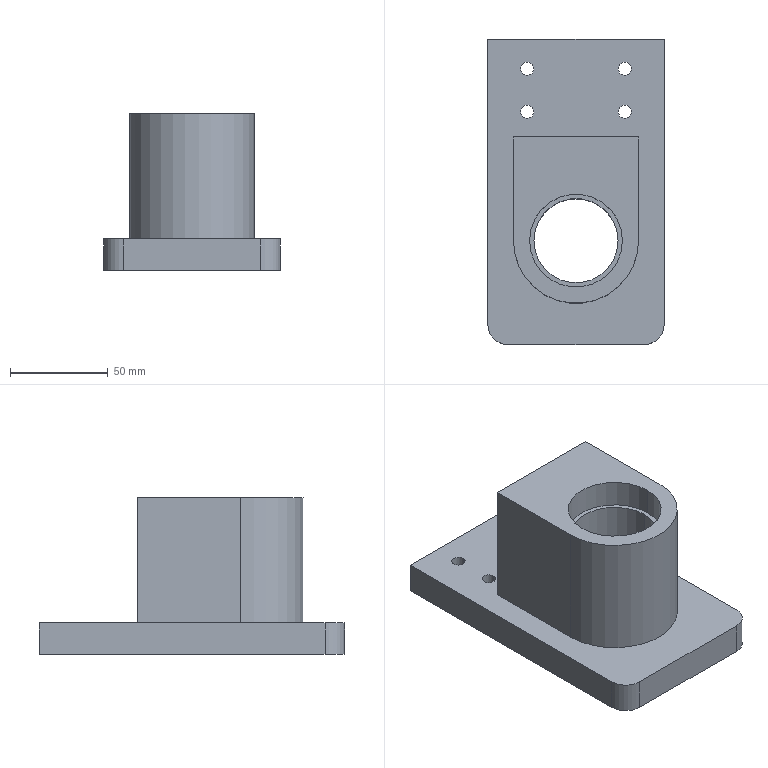NC program | NX | posted with a generic post | part box 90 x 156 x 80 mm
Lines 1 to 1164 of 8711:
N10 G17 G21 G94 G90
(CAVITY_MILL_COPY , TOOL : 刀杆C25-D25-150-2T)
N12 T01 M6
N14 G53
N16 G17 G0 G90 X-98.941 Y0. S2000 M3
N18 G43 Z30. H1
N20 Z1.5
N22 G94 G1 Z-0.5 F3000.
N24 X-82.691
N26 Y48.791
N28 X-82.682 Y50.031
N30 G2 X-81.523 Y51.183 R1.159
N32 G1 X81.523
N34 G2 X82.682 Y50.031 R1.159
N36 G1 X82.691 Y48.791
N38 Y28.521
N40 X63.971
N42 G3 X60.754 Y32.463 R48.293
N44 G1 X63.971
N46 Y28.521
N48 X70.565 Y17.419
N50 X63.971 Y28.521
N52 X82.691
N54 Y-48.791
N56 X82.682 Y-50.031
N58 G2 X81.523 Y-51.183 R1.159
N60 G1 X60.754
N62 Y-32.463
N64 G3 X63.971 Y-28.521 R48.293
N66 G1 X70.565 Y-17.419
N68 X63.971 Y-28.521
N70 Y-32.463
N72 X60.754
N74 Y-51.183
N76 X-81.523
N78 G2 X-82.682 Y-50.031 R1.159
N80 G1 X-82.691 Y-48.791
N82 Y0.
N84 X-63.971
N86 Y32.463
N88 X-44.264
N90 G3 X-44.293 Y32. R3.744
N92 G1 Y-32.
N94 G3 X-44.264 Y-32.463 R3.744
N96 G1 X-40.549 Y-32.
N98 Y32.
N100 X-40.532 Y32.037
N102 X-40.47 Y33.362
N104 G2 X-28. Y44.549 R12.555
N106 G1 X25.
N108 G2 X69.549 Y0. R44.549
N110 X25. Y-44.549 R44.549
N112 G1 X-28.
N114 G2 X-40.47 Y-33.362 R12.555
N116 G1 X-40.532 Y-32.037
N118 X-40.549 Y-32.
N120 X-44.264 Y-32.463
N122 X-63.971
N124 Y0.
N126 X-98.941
N128 Z1.5
N130 G0 Z30.
N132 X35.297 Y-4.41
N134 Z3.
N136 G2 X25. Y-11.201 Z-0.5 R11.201
N138 X13.799 Y0. R11.201
N140 X25. Y-11.201 R-11.201
N142 G1 Z1.5
N144 G0 Z2.5
N146 X35.273 Y-4.335
N148 G2 X25. Y-11.15 Z-1. R11.15
N150 X13.85 Y0. R11.15
N152 X25. Y-11.15 R-11.15
N154 G1 Z1.
N156 G0 Z30.
N158 X-98.999 Y0.
N160 Z1.
N162 G1 Z-1.
N164 X-82.749
N166 Y48.795
N168 X-82.741 Y50.036
N170 G2 X-81.528 Y51.242 R1.214
N172 G1 X81.528
N174 G2 X82.741 Y50.036 R1.214
N176 G1 X82.749 Y48.796
N178 Y28.529
N180 X64.029
N182 G3 X60.769 Y32.522 R48.344
N184 G1 X64.029
N186 Y28.529
N188 X70.622 Y17.419
N190 X64.029 Y28.529
N192 X82.749
N194 Y-48.795
N196 X82.741 Y-50.036
N198 G2 X81.528 Y-51.242 R1.214
N200 G1 X60.769
N202 Y-32.522
N204 G3 X64.029 Y-28.528 R48.344
N206 G1 X70.622 Y-17.419
N208 X64.029 Y-28.528
N210 Y-32.522
N212 X60.769
N214 Y-51.242
N216 X-81.528
N218 G2 X-82.741 Y-50.036 R1.214
N220 G1 X-82.749 Y-48.796
N222 Y0.
N224 X-64.029
N226 Y32.522
N228 X-44.336
N230 G3 X-44.344 Y32. R16.344
N232 G1 Y-32.
N234 G3 X-44.336 Y-32.522 R16.344
N236 G1 X-40.594 Y-32.403
N238 G2 X-40.6 Y-32. R12.6
N240 G1 Y32.
N242 G2 X-28. Y44.6 R12.6
N244 G1 X25.
N246 G2 X69.6 Y0. R44.6
N248 X25. Y-44.6 R44.6
N250 G1 X-28.
N252 G2 X-40.594 Y-32.403 R12.6
N254 G1 X-44.336 Y-32.522
N256 X-64.029
N258 Y0.
N260 X-98.999
N262 Z1.
N264 G0 Z1.5
N266 Z0.5
N268 G1 Z-1.5
N270 X-82.749
N272 X-82.75 Y48.793
N274 X-82.741 Y50.037
N276 G2 X-81.528 Y51.242 R1.214
N278 G1 X81.528
N280 G2 X82.741 Y50.036 R1.214
N282 G1 X82.749 Y48.795
N284 Y28.529
N286 X64.029
N288 G3 X60.769 Y32.522 R48.344
N290 G1 X64.029
N292 Y28.529
N294 X70.622 Y17.419
N296 X64.029 Y28.529
N298 X82.749
N300 X82.75 Y-48.793
N302 X82.741 Y-50.037
N304 G2 X81.528 Y-51.242 R1.214
N306 G1 X60.769
N308 Y-32.522
N310 G3 X64.029 Y-28.528 R48.344
N312 G1 X70.622 Y-17.418
N314 X64.029 Y-28.528
N316 Y-32.522
N318 X60.769
N320 Y-51.242
N322 X-81.528
N324 G2 X-82.741 Y-50.036 R1.214
N326 G1 X-82.749 Y-48.795
N328 Y0.
N330 X-64.029
N332 Y32.522
N334 X-44.336
N336 G3 X-44.344 Y32. R16.344
N338 G1 Y-32.
N340 G3 X-44.336 Y-32.522 R16.344
N342 G1 X-40.594 Y-32.403
N344 G2 X-40.6 Y-32. R12.6
N346 G1 Y32.
N348 G2 X-28. Y44.6 R12.6
N350 G1 X25.
N352 G2 X69.6 Y0. R44.6
N354 X25. Y-44.6 R44.6
N356 G1 X-28.
N358 G2 X-40.594 Y-32.403 R12.6
N360 G1 X-44.336 Y-32.522
N362 X-64.029
N364 Y0.
N366 X-98.999
N368 Z0.5
N370 G0 Z30.
N372 X35.273 Y-4.335
N374 Z2.
N376 G2 X25. Y-11.15 Z-1.5 R11.15
N378 X13.85 Y0. R11.15
N380 X25. Y-11.15 R-11.15
N382 G1 Z0.5
N384 G0 Z1.5
N386 X35.273 Y-4.335
N388 G2 X25. Y-11.15 Z-2. R11.15
N390 X13.85 Y0. R11.15
N392 X25. Y-11.15 R-11.15
N394 G1 Z0.
N396 G0 Z30.
N398 X-98.999 Y0.
N400 Z0.
N402 G1 Z-2.
N404 X-82.749
N406 X-82.75 Y48.792
N408 X-82.741 Y50.037
N410 G2 X-81.528 Y51.242 R1.214
N412 G1 X81.527
N414 G2 X82.738 Y50.031 R1.211
N416 G1 X82.741 Y28.542
N418 X64.021 Y28.54
N420 G3 X60.769 Y32.522 R48.344
N422 G1 X64.02
N424 X64.021 Y28.54
N426 X70.615 Y17.434
N428 X64.021 Y28.54
N430 X82.741 Y28.542
N432 X82.75 Y-49.859
N434 G2 X82.732 Y-50.169 R2.637
N436 X81.524 Y-51.242 R1.216
N438 G1 X60.769
N440 Y-32.522
N442 G3 X64.028 Y-28.53 R48.344
N444 G1 X70.62 Y-17.423
N446 X64.028 Y-28.53
N448 Y-32.522
N450 X60.769
N452 Y-51.242
N454 X-81.528
N456 G2 X-82.741 Y-50.036 R1.214
N458 G1 X-82.749 Y-48.795
N460 Y0.
N462 X-64.029
N464 X-64.03 Y32.522
N466 X-44.336
N468 G3 X-44.344 Y32. R16.344
N470 G1 Y-32.
N472 G3 X-44.336 Y-32.522 R16.344
N474 G1 X-40.594 Y-32.403
N476 G2 X-40.6 Y-32. R12.6
N478 G1 Y32.
N480 G2 X-28. Y44.6 R12.6
N482 G1 X25.
N484 G2 X69.6 Y0. R44.6
N486 X25. Y-44.6 R44.6
N488 G1 X-28.
N490 G2 X-40.594 Y-32.403 R12.6
N492 G1 X-44.336 Y-32.522
N494 X-64.029
N496 Y0.
N498 X-98.999
N500 Z0.
N502 G0 Z0.5
N504 Z-0.5
N506 G1 Z-2.5
N508 X-82.749
N510 X-82.75 Y48.792
N512 X-82.741 Y50.037
N514 G2 X-81.528 Y51.242 R1.214
N516 G1 X81.527
N518 G2 X82.738 Y50.031 R1.211
N520 G1 X82.741 Y28.542
N522 X64.021 Y28.54
N524 G3 X60.769 Y32.522 R48.344
N526 G1 X64.02
N528 X64.021 Y28.54
N530 X70.615 Y17.434
N532 X64.021 Y28.54
N534 X82.741 Y28.542
N536 X82.75 Y-49.859
N538 G2 X82.732 Y-50.169 R2.637
N540 X81.524 Y-51.242 R1.216
N542 G1 X60.769
N544 Y-32.522
N546 G3 X64.028 Y-28.53 R48.344
N548 G1 X70.62 Y-17.423
N550 X64.028 Y-28.53
N552 Y-32.522
N554 X60.769
N556 Y-51.242
N558 X-81.528
N560 G2 X-82.741 Y-50.036 R1.214
N562 G1 X-82.749 Y-48.795
N564 Y0.
N566 X-64.029
N568 X-64.03 Y32.522
N570 X-44.336
N572 G3 X-44.344 Y32. R16.344
N574 G1 Y-32.
N576 G3 X-44.336 Y-32.522 R16.344
N578 G1 X-40.594 Y-32.403
N580 G2 X-40.6 Y-32. R12.6
N582 G1 Y32.
N584 G2 X-28. Y44.6 R12.6
N586 G1 X25.
N588 G2 X69.6 Y0. R44.6
N590 X25. Y-44.6 R44.6
N592 G1 X-28.
N594 G2 X-40.594 Y-32.403 R12.6
N596 G1 X-44.336 Y-32.522
N598 X-64.029
N600 Y0.
N602 X-98.999
N604 Z-0.5
N606 G0 Z30.
N608 X35.273 Y-4.335
N610 Z1.
N612 G2 X25. Y-11.15 Z-2.5 R11.15
N614 X13.85 Y0. R11.15
N616 X25. Y-11.15 R-11.15
N618 G1 Z-0.5
N620 G0 Z0.5
N622 X35.273 Y-4.335
N624 G2 X25. Y-11.15 Z-3. R11.15
N626 X13.85 Y0. R11.15
N628 X25. Y-11.15 R-11.15
N630 G1 Z-1.
N632 G0 Z30.
N634 X-98.988 Y0.
N636 Z-1.
N638 G1 Z-3.
N640 X-82.738
N642 Y50.031
N644 G2 X-81.527 Y51.242 R1.211
N646 G1 X81.527
N648 G2 X82.738 Y50.031 R1.211
N650 G1 X82.741 Y28.542
N652 X64.021 Y28.54
N654 G3 X60.769 Y32.522 R48.344
N656 G1 X64.02
N658 X64.021 Y28.54
N660 X70.615 Y17.434
N662 X64.021 Y28.54
N664 X82.741 Y28.542
N666 X82.75 Y-49.859
N668 G2 X82.732 Y-50.169 R2.637
N670 X81.524 Y-51.242 R1.216
N672 G1 X60.769
N674 Y-32.522
N676 G3 X64.028 Y-28.53 R48.344
N678 G1 X70.62 Y-17.423
N680 X64.028 Y-28.53
N682 Y-32.522
N684 X60.769
N686 Y-51.242
N688 X-81.527
N690 G2 X-82.738 Y-50.031 R1.211
N692 G1 Y0.
N694 X-64.018
N696 Y32.522
N698 X-44.336
N700 G3 X-44.344 Y32. R16.344
N702 G1 Y-32.
N704 G3 X-44.336 Y-32.522 R16.344
N706 G1 X-40.594 Y-32.403
N708 G2 X-40.6 Y-32. R12.6
N710 G1 Y32.
N712 G2 X-28. Y44.6 R12.6
N714 G1 X25.
N716 G2 X69.6 Y0. R44.6
N718 X25. Y-44.6 R44.6
N720 G1 X-28.
N722 G2 X-40.594 Y-32.403 R12.6
N724 G1 X-44.336 Y-32.522
N726 X-64.018
N728 Y0.
N730 X-98.988
N732 Z-1.
N734 G0 Z-0.5
N736 Z-1.5
N738 G1 Z-3.5
N740 X-82.738
N742 Y50.031
N744 G2 X-81.527 Y51.242 R1.211
N746 G1 X81.527
N748 G2 X82.738 Y50.031 R1.211
N750 G1 X82.741 Y28.542
N752 X64.021 Y28.54
N754 G3 X60.769 Y32.522 R48.344
N756 G1 X64.02
N758 X64.021 Y28.54
N760 X70.615 Y17.434
N762 X64.021 Y28.54
N764 X82.741 Y28.542
N766 X82.75 Y-49.859
N768 G2 X82.732 Y-50.169 R2.637
N770 X81.524 Y-51.242 R1.216
N772 G1 X60.769
N774 Y-32.522
N776 G3 X64.028 Y-28.53 R48.344
N778 G1 X70.62 Y-17.423
N780 X64.028 Y-28.53
N782 Y-32.522
N784 X60.769
N786 Y-51.242
N788 X-81.527
N790 G2 X-82.738 Y-50.031 R1.211
N792 G1 Y0.
N794 X-64.018
N796 Y32.522
N798 X-44.336
N800 G3 X-44.344 Y32. R16.344
N802 G1 Y-32.
N804 G3 X-44.336 Y-32.522 R16.344
N806 G1 X-40.594 Y-32.403
N808 G2 X-40.6 Y-32. R12.6
N810 G1 Y32.
N812 G2 X-28. Y44.6 R12.6
N814 G1 X25.
N816 G2 X69.6 Y0. R44.6
N818 X25. Y-44.6 R44.6
N820 G1 X-28.
N822 G2 X-40.594 Y-32.403 R12.6
N824 G1 X-44.336 Y-32.522
N826 X-64.018
N828 Y0.
N830 X-98.988
N832 Z-1.5
N834 G0 Z30.
N836 X35.273 Y-4.335
N838 Z0.
N840 G2 X25. Y-11.15 Z-3.5 R11.15
N842 X13.85 Y0. R11.15
N844 X25. Y-11.15 R-11.15
N846 G1 Z-1.5
N848 G0 Z-0.5
N850 X35.273 Y-4.335
N852 G2 X25. Y-11.15 Z-4. R11.15
N854 X13.85 Y0. R11.15
N856 X25. Y-11.15 R-11.15
N858 G1 Z-2.
N860 G0 Z30.
N862 X-98.999 Y0.
N864 Z-2.
N866 G1 Z-4.
N868 X-82.749
N870 X-82.75 Y48.792
N872 X-82.741 Y50.037
N874 G2 X-81.528 Y51.242 R1.214
N876 G1 X81.528
N878 G2 X82.741 Y50.036 R1.214
N880 G1 X82.749 Y48.795
N882 Y28.529
N884 X64.029 Y28.528
N886 G3 X60.769 Y32.522 R48.344
N888 G1 X64.029
N890 Y28.528
N892 X70.622 Y17.418
N894 X64.029 Y28.528
N896 X82.749 Y28.529
N898 X82.75 Y-48.792
N900 X82.741 Y-50.037
N902 G2 X81.528 Y-51.242 R1.214
N904 G1 X60.769
N906 Y-32.522
N908 G3 X64.03 Y-28.528 R48.344
N910 G1 X70.622 Y-17.417
N912 X64.03 Y-28.528
N914 Y-32.522
N916 X60.769
N918 Y-51.242
N920 X-81.528
N922 G2 X-82.741 Y-50.036 R1.214
N924 G1 X-82.749 Y-48.795
N926 Y0.
N928 X-64.029
N930 X-64.03 Y32.522
N932 X-44.336
N934 G3 X-44.344 Y32. R16.344
N936 G1 Y-32.
N938 G3 X-44.336 Y-32.522 R16.344
N940 G1 X-40.594 Y-32.403
N942 G2 X-40.6 Y-32. R12.6
N944 G1 Y32.
N946 G2 X-28. Y44.6 R12.6
N948 G1 X25.
N950 G2 X69.6 Y0. R44.6
N952 X25. Y-44.6 R44.6
N954 G1 X-28.
N956 G2 X-40.594 Y-32.403 R12.6
N958 G1 X-44.336 Y-32.522
N960 X-64.029
N962 Y0.
N964 X-98.999
N966 Z-2.
N968 G0 Z-1.5
N970 Z-2.5
N972 G1 Z-4.5
N974 X-82.749
N976 X-82.75 Y48.792
N978 X-82.741 Y50.037
N980 G2 X-81.528 Y51.242 R1.214
N982 G1 X81.528
N984 G2 X82.741 Y50.036 R1.214
N986 G1 X82.749 Y48.795
N988 Y28.529
N990 X64.029 Y28.528
N992 G3 X60.769 Y32.522 R48.344
N994 G1 X64.029
N996 Y28.528
N998 X70.622 Y17.418
N1000 X64.029 Y28.528
N1002 X82.749 Y28.529
N1004 X82.75 Y-48.792
N1006 X82.741 Y-50.037
N1008 G2 X81.528 Y-51.242 R1.214
N1010 G1 X60.769
N1012 Y-32.522
N1014 G3 X64.03 Y-28.528 R48.344
N1016 G1 X70.622 Y-17.417
N1018 X64.03 Y-28.528
N1020 Y-32.522
N1022 X60.769
N1024 Y-51.242
N1026 X-81.528
N1028 G2 X-82.741 Y-50.036 R1.214
N1030 G1 X-82.749 Y-48.795
N1032 Y0.
N1034 X-64.029
N1036 X-64.03 Y32.522
N1038 X-44.336
N1040 G3 X-44.344 Y32. R16.344
N1042 G1 Y-32.
N1044 G3 X-44.336 Y-32.522 R16.344
N1046 G1 X-40.594 Y-32.403
N1048 G2 X-40.6 Y-32. R12.6
N1050 G1 Y32.
N1052 G2 X-28. Y44.6 R12.6
N1054 G1 X25.
N1056 G2 X69.6 Y0. R44.6
N1058 X25. Y-44.6 R44.6
N1060 G1 X-28.
N1062 G2 X-40.594 Y-32.403 R12.6
N1064 G1 X-44.336 Y-32.522
N1066 X-64.029
N1068 Y0.
N1070 X-98.999
N1072 Z-2.5
N1074 G0 Z30.
N1076 X35.273 Y-4.335
N1078 Z-1.
N1080 G2 X25. Y-11.15 Z-4.5 R11.15
N1082 X13.85 Y0. R11.15
N1084 X25. Y-11.15 R-11.15
N1086 G1 Z-2.5
N1088 G0 Z-1.5
N1090 X35.273 Y-4.335
N1092 G2 X25. Y-11.15 Z-5. R11.15
N1094 X13.85 Y0. R11.15
N1096 X25. Y-11.15 R-11.15
N1098 G1 Z-3.
N1100 G0 Z30.
N1102 X-98.999 Y0.
N1104 Z-3.
N1106 G1 Z-5.
N1108 X-82.749
N1110 X-82.75 Y48.792
N1112 X-82.741 Y50.037
N1114 G2 X-81.528 Y51.242 R1.214
N1116 G1 X81.528
N1118 G2 X82.741 Y50.036 R1.214
N1120 G1 X82.749 Y48.795
N1122 Y28.529
N1124 X64.029 Y28.528
N1126 G3 X60.769 Y32.522 R48.344
N1128 G1 X64.029
N1130 Y28.528
N1132 X70.622 Y17.418
N1134 X64.029 Y28.528
N1136 X82.749 Y28.529
N1138 X82.75 Y-48.792
N1140 X82.741 Y-50.037
N1142 G2 X81.528 Y-51.242 R1.214
N1144 G1 X60.769
N1146 Y-32.522
N1148 G3 X64.03 Y-28.528 R48.344
N1150 G1 X70.622 Y-17.417
N1152 X64.03 Y-28.528
N1154 Y-32.522
N1156 X60.769
N1158 Y-51.242
N1160 X-81.528
N1162 G2 X-82.741 Y-50.036 R1.214
N1164 G1 X-82.749 Y-48.795
N1166 Y0.
N1168 X-64.029
N1170 X-64.03 Y32.522
N1172 X-44.336
N1174 G3 X-44.344 Y32. R16.344
N1176 G1 Y-32.
N1178 G3 X-44.336 Y-32.522 R16.344
N1180 G1 X-40.594 Y-32.403
N1182 G2 X-40.6 Y-32. R12.6
N1184 G1 Y32.
N1186 G2 X-28. Y44.6 R12.6
N1188 G1 X25.
N1190 G2 X69.6 Y0. R44.6
N1192 X25. Y-44.6 R44.6
N1194 G1 X-28.
N1196 G2 X-40.594 Y-32.403 R12.6
N1198 G1 X-44.336 Y-32.522
N1200 X-64.029
N1202 Y0.
N1204 X-98.999
N1206 Z-3.
N1208 G0 Z-2.5
N1210 Z-3.5
N1212 G1 Z-5.5
N1214 X-82.749
N1216 X-82.75 Y48.792
N1218 X-82.741 Y50.037
N1220 G2 X-81.528 Y51.242 R1.214
N1222 G1 X81.528
N1224 G2 X82.741 Y50.036 R1.214
N1226 G1 X82.749 Y48.795
N1228 Y28.529
N1230 X64.029 Y28.528
N1232 G3 X60.769 Y32.522 R48.344
N1234 G1 X64.029
N1236 Y28.528
N1238 X70.622 Y17.418
N1240 X64.029 Y28.528
N1242 X82.749 Y28.529
N1244 X82.75 Y-48.792
N1246 X82.741 Y-50.037
N1248 G2 X81.528 Y-51.242 R1.214
N1250 G1 X60.769
N1252 Y-32.522
N1254 G3 X64.03 Y-28.528 R48.344
N1256 G1 X70.622 Y-17.417
N1258 X64.03 Y-28.528
N1260 Y-32.522
N1262 X60.769
N1264 Y-51.242
N1266 X-81.528
N1268 G2 X-82.741 Y-50.036 R1.214
N1270 G1 X-82.749 Y-48.795
N1272 Y0.
N1274 X-64.029
N1276 X-64.03 Y32.522
N1278 X-44.336
N1280 G3 X-44.344 Y32. R16.344
N1282 G1 Y-32.
N1284 G3 X-44.336 Y-32.522 R16.344
N1286 G1 X-40.594 Y-32.403
N1288 G2 X-40.6 Y-32. R12.6
N1290 G1 Y32.
N1292 G2 X-28. Y44.6 R12.6
N1294 G1 X25.
N1296 G2 X69.6 Y0. R44.6
N1298 X25. Y-44.6 R44.6
N1300 G1 X-28.
N1302 G2 X-40.594 Y-32.403 R12.6
N1304 G1 X-44.336 Y-32.522
N1306 X-64.029
N1308 Y0.
N1310 X-98.999
N1312 Z-3.5
N1314 G0 Z30.
N1316 X35.273 Y-4.335
N1318 Z-2.
N1320 G2 X25. Y-11.15 Z-5.5 R11.15
N1322 X13.85 Y0. R11.15
N1324 X25. Y-11.15 R-11.15
N1326 G1 Z-3.5
N1328 G0 Z-2.5
N1330 X35.273 Y-4.335
N1332 G2 X25. Y-11.15 Z-6. R11.15
N1334 X13.85 Y0. R11.15
N1336 X25. Y-11.15 R-11.15
N1338 G1 Z-4.
N1340 G0 Z30.
N1342 X-98.999 Y0.
N1344 Z-4.
N1346 G1 Z-6.
N1348 X-82.749
N1350 X-82.75 Y48.792
N1352 X-82.741 Y50.037
N1354 G2 X-81.528 Y51.242 R1.214
N1356 G1 X81.528
N1358 G2 X82.741 Y50.036 R1.214
N1360 G1 X82.749 Y48.795
N1362 Y28.529
N1364 X64.029 Y28.528
N1366 G3 X60.769 Y32.522 R48.344
N1368 G1 X64.029
N1370 Y28.528
N1372 X70.622 Y17.418
N1374 X64.029 Y28.528
N1376 X82.749 Y28.529
N1378 X82.75 Y-48.792
N1380 X82.741 Y-50.037
N1382 G2 X81.528 Y-51.242 R1.214
N1384 G1 X60.769
N1386 Y-32.522
N1388 G3 X64.03 Y-28.527 R48.344
N1390 G1 X70.622 Y-17.417
N1392 X64.03 Y-28.527
N1394 Y-32.522
N1396 X60.769
N1398 Y-51.242
N1400 X-81.528
N1402 G2 X-82.741 Y-50.036 R1.214
N1404 G1 X-82.749 Y-48.795
N1406 Y0.
N1408 X-64.029
N1410 X-64.03 Y32.522
N1412 X-44.336
N1414 G3 X-44.344 Y32. R16.344
N1416 G1 Y-32.
N1418 G3 X-44.336 Y-32.522 R16.344
N1420 G1 X-40.594 Y-32.403
N1422 G2 X-40.6 Y-32. R12.6
N1424 G1 Y32.
N1426 G2 X-28. Y44.6 R12.6
N1428 G1 X25.
N1430 G2 X69.6 Y0. R44.6
N1432 X25. Y-44.6 R44.6
N1434 G1 X-28.
N1436 G2 X-40.594 Y-32.403 R12.6
N1438 G1 X-44.336 Y-32.522
N1440 X-64.029
N1442 Y0.
N1444 X-98.999
N1446 Z-4.
N1448 G0 Z-3.5
N1450 Z-4.5
N1452 G1 Z-6.5
N1454 X-82.749
N1456 X-82.75 Y48.792
N1458 X-82.741 Y50.037
N1460 G2 X-81.528 Y51.242 R1.214
N1462 G1 X81.528
N1464 G2 X82.741 Y50.036 R1.214
N1466 G1 X82.749 Y48.795
N1468 Y28.529
N1470 X64.029 Y28.528
N1472 G3 X60.769 Y32.522 R48.344
N1474 G1 X64.029
N1476 Y28.528
N1478 X70.622 Y17.418
N1480 X64.029 Y28.528
N1482 X82.749 Y28.529
N1484 X82.75 Y-48.792
N1486 X82.741 Y-50.037
N1488 G2 X81.528 Y-51.242 R1.214
N1490 G1 X60.769
N1492 Y-32.522
N1494 G3 X64.03 Y-28.527 R48.344
N1496 G1 X70.622 Y-17.417
N1498 X64.03 Y-28.527
N1500 Y-32.522
N1502 X60.769
N1504 Y-51.242
N1506 X-81.528
N1508 G2 X-82.741 Y-50.036 R1.214
N1510 G1 X-82.749 Y-48.795
N1512 Y0.
N1514 X-64.029
N1516 X-64.03 Y32.522
N1518 X-44.336
N1520 G3 X-44.344 Y32. R16.344
N1522 G1 Y-32.
N1524 G3 X-44.336 Y-32.522 R16.344
N1526 G1 X-40.594 Y-32.403
N1528 G2 X-40.6 Y-32. R12.6
N1530 G1 Y32.
N1532 G2 X-28. Y44.6 R12.6
N1534 G1 X25.
N1536 G2 X69.6 Y0. R44.6
N1538 X25. Y-44.6 R44.6
N1540 G1 X-28.
N1542 G2 X-40.594 Y-32.403 R12.6
N1544 G1 X-44.336 Y-32.522
N1546 X-64.029
N1548 Y0.
N1550 X-98.999
N1552 Z-4.5
N1554 G0 Z30.
N1556 X35.273 Y-4.335
N1558 Z-3.
N1560 G2 X25. Y-11.15 Z-6.5 R11.15
N1562 X13.85 Y0. R11.15
N1564 X25. Y-11.15 R-11.15
N1566 G1 Z-4.5
N1568 G0 Z-3.5
N1570 X35.273 Y-4.335
N1572 G2 X25. Y-11.15 Z-7. R11.15
N1574 X13.85 Y0. R11.15
N1576 X25. Y-11.15 R-11.15
N1578 G1 Z-5.
N1580 G0 Z30.
N1582 X-98.999 Y0.
N1584 Z-5.
N1586 G1 Z-7.
N1588 X-82.749
N1590 X-82.75 Y48.792
N1592 X-82.741 Y50.037
N1594 G2 X-81.528 Y51.242 R1.214
N1596 G1 X81.527
N1598 G2 X82.741 Y50.036 R1.214
N1600 G1 X82.749 Y48.795
N1602 Y28.529
N1604 X64.029 Y28.528
N1606 G3 X60.769 Y32.522 R48.344
N1608 G1 X64.029
N1610 Y28.528
N1612 X70.622 Y17.418
N1614 X64.029 Y28.528
N1616 X82.749 Y28.529
N1618 X82.75 Y-48.792
N1620 X82.741 Y-50.037
N1622 G2 X81.528 Y-51.242 R1.214
N1624 G1 X60.769
N1626 Y-32.522
N1628 G3 X64.03 Y-28.527 R48.344
N1630 G1 X70.622 Y-17.417
N1632 X64.03 Y-28.527
N1634 Y-32.522
N1636 X60.769
N1638 Y-51.242
N1640 X-81.527
N1642 G2 X-82.741 Y-50.036 R1.214
N1644 G1 X-82.749 Y-48.795
N1646 Y0.
N1648 X-64.029
N1650 X-64.03 Y32.522
N1652 X-44.336
N1654 G3 X-44.344 Y32. R16.344
N1656 G1 Y-32.
N1658 G3 X-44.336 Y-32.522 R16.344
N1660 G1 X-40.594 Y-32.403
N1662 G2 X-40.6 Y-32. R12.6
N1664 G1 Y32.
N1666 G2 X-28. Y44.6 R12.6
N1668 G1 X25.
N1670 G2 X69.6 Y0. R44.6
N1672 X25. Y-44.6 R44.6
N1674 G1 X-28.
N1676 G2 X-40.594 Y-32.403 R12.6
N1678 G1 X-44.336 Y-32.522
N1680 X-64.029
N1682 Y0.
N1684 X-98.999
N1686 Z-5.
N1688 G0 Z-4.5
N1690 Z-5.5
N1692 G1 Z-7.5
N1694 X-82.749
N1696 X-82.75 Y48.792
N1698 X-82.741 Y50.037
N1700 G2 X-81.528 Y51.242 R1.214
N1702 G1 X81.527
N1704 G2 X82.741 Y50.036 R1.214
N1706 G1 X82.749 Y48.795
N1708 Y28.529
N1710 X64.029 Y28.528
N1712 G3 X60.769 Y32.522 R48.344
N1714 G1 X64.029
N1716 Y28.528
N1718 X70.622 Y17.418
N1720 X64.029 Y28.528
N1722 X82.749 Y28.529
N1724 X82.75 Y-48.792
N1726 X82.741 Y-50.037
N1728 G2 X81.528 Y-51.242 R1.214
N1730 G1 X60.769
N1732 Y-32.522
N1734 G3 X64.03 Y-28.527 R48.344
N1736 G1 X70.622 Y-17.417
N1738 X64.03 Y-28.527
N1740 Y-32.522
N1742 X60.769
N1744 Y-51.242
N1746 X-81.527
N1748 G2 X-82.741 Y-50.036 R1.214
N1750 G1 X-82.749 Y-48.795
N1752 Y0.
N1754 X-64.029
N1756 X-64.03 Y32.522
N1758 X-44.336
N1760 G3 X-44.344 Y32. R16.344
N1762 G1 Y-32.
N1764 G3 X-44.336 Y-32.522 R16.344
N1766 G1 X-40.594 Y-32.403
N1768 G2 X-40.6 Y-32. R12.6
N1770 G1 Y32.
N1772 G2 X-28. Y44.6 R12.6
N1774 G1 X25.
N1776 G2 X69.6 Y0. R44.6
N1778 X25. Y-44.6 R44.6
N1780 G1 X-28.
N1782 G2 X-40.594 Y-32.403 R12.6
N1784 G1 X-44.336 Y-32.522
N1786 X-64.029
N1788 Y0.
N1790 X-98.999
N1792 Z-5.5
N1794 G0 Z30.
N1796 X35.273 Y-4.335
N1798 Z-4.
N1800 G2 X25. Y-11.15 Z-7.5 R11.15
N1802 X13.85 Y0. R11.15
N1804 X25. Y-11.15 R-11.15
N1806 G1 Z-5.5
N1808 G0 Z-4.5
N1810 X35.273 Y-4.335
N1812 G2 X25. Y-11.15 Z-8. R11.15
N1814 X13.85 Y0. R11.15
N1816 X25. Y-11.15 R-11.15
N1818 G1 Z-6.
N1820 G0 Z30.
N1822 X-98.999 Y0.
N1824 Z-6.
N1826 G1 Z-8.
N1828 X-82.749
N1830 X-82.75 Y48.792
N1832 X-82.741 Y50.037
N1834 G2 X-81.528 Y51.242 R1.214
N1836 G1 X81.527
N1838 G2 X82.741 Y50.036 R1.214
N1840 G1 X82.749 Y48.795
N1842 Y28.529
N1844 X64.029 Y28.528
N1846 G3 X60.769 Y32.522 R48.344
N1848 G1 X64.029
N1850 Y28.528
N1852 X70.622 Y17.418
N1854 X64.029 Y28.528
N1856 X82.749 Y28.529
N1858 X82.75 Y-48.792
N1860 X82.741 Y-50.037
N1862 G2 X81.528 Y-51.242 R1.214
N1864 G1 X60.769
N1866 Y-32.522
N1868 G3 X64.03 Y-28.527 R48.344
N1870 G1 X70.622 Y-17.417
N1872 X64.03 Y-28.527
N1874 Y-32.522
N1876 X60.769
N1878 Y-51.242
N1880 X-81.527
N1882 G2 X-82.741 Y-50.036 R1.214
N1884 G1 X-82.749 Y-48.795
N1886 Y0.
N1888 X-64.029
N1890 X-64.03 Y32.522
N1892 X-44.336
N1894 G3 X-44.344 Y32. R16.344
N1896 G1 Y-32.
N1898 G3 X-44.336 Y-32.522 R16.344
N1900 G1 X-40.594 Y-32.403
N1902 G2 X-40.6 Y-32. R12.6
N1904 G1 Y32.
N1906 G2 X-28. Y44.6 R12.6
N1908 G1 X25.
N1910 G2 X69.6 Y0. R44.6
N1912 X25. Y-44.6 R44.6
N1914 G1 X-28.
N1916 G2 X-40.594 Y-32.403 R12.6
N1918 G1 X-44.336 Y-32.522
N1920 X-64.029
N1922 Y0.
N1924 X-98.999
N1926 Z-6.
N1928 G0 Z-5.5
N1930 Z-6.5
N1932 G1 Z-8.5
N1934 X-82.749
N1936 X-82.75 Y48.792
N1938 X-82.741 Y50.037
N1940 G2 X-81.528 Y51.242 R1.214
N1942 G1 X81.527
N1944 G2 X82.741 Y50.036 R1.214
N1946 G1 X82.749 Y48.795
N1948 Y28.529
N1950 X64.029 Y28.528
N1952 G3 X60.769 Y32.522 R48.344
N1954 G1 X64.029
N1956 Y28.528
N1958 X70.622 Y17.418
N1960 X64.029 Y28.528
N1962 X82.749 Y28.529
N1964 X82.75 Y-48.792
N1966 X82.741 Y-50.037
N1968 G2 X81.528 Y-51.242 R1.214
N1970 G1 X60.769
N1972 Y-32.522
N1974 G3 X64.03 Y-28.527 R48.344
N1976 G1 X70.622 Y-17.417
N1978 X64.03 Y-28.527
N1980 Y-32.522
N1982 X60.769
N1984 Y-51.242
N1986 X-81.527
N1988 G2 X-82.741 Y-50.036 R1.214
N1990 G1 X-82.749 Y-48.795
N1992 Y0.
N1994 X-64.029
N1996 X-64.03 Y32.522
N1998 X-44.336
N2000 G3 X-44.344 Y32. R16.344
N2002 G1 Y-32.
N2004 G3 X-44.336 Y-32.522 R16.344
N2006 G1 X-40.594 Y-32.403
N2008 G2 X-40.6 Y-32. R12.6
N2010 G1 Y32.
N2012 G2 X-28. Y44.6 R12.6
N2014 G1 X25.
N2016 G2 X69.6 Y0. R44.6
N2018 X25. Y-44.6 R44.6
N2020 G1 X-28.
N2022 G2 X-40.594 Y-32.403 R12.6
N2024 G1 X-44.336 Y-32.522
N2026 X-64.029
N2028 Y0.
N2030 X-98.999
N2032 Z-6.5
N2034 G0 Z30.
N2036 X35.273 Y-4.335
N2038 Z-5.
N2040 G2 X25. Y-11.15 Z-8.5 R11.15
N2042 X13.85 Y0. R11.15
N2044 X25. Y-11.15 R-11.15
N2046 G1 Z-6.5
N2048 G0 Z-5.5
N2050 X35.273 Y-4.335
N2052 G2 X25. Y-11.15 Z-9. R11.15
N2054 X13.85 Y0. R11.15
N2056 X25. Y-11.15 R-11.15
N2058 G1 Z-7.
N2060 G0 Z30.
N2062 X-98.999 Y0.
N2064 Z-7.
N2066 G1 Z-9.
N2068 X-82.749
N2070 X-82.75 Y48.792
N2072 X-82.741 Y50.037
N2074 G2 X-81.528 Y51.242 R1.214
N2076 G1 X81.527
N2078 G2 X82.741 Y50.036 R1.214
N2080 G1 X82.749 Y48.795
N2082 Y28.529
N2084 X64.029 Y28.528
N2086 G3 X60.769 Y32.522 R48.344
N2088 G1 X64.029
N2090 Y28.528
N2092 X70.622 Y17.418
N2094 X64.029 Y28.528
N2096 X82.749 Y28.529
N2098 X82.75 Y-48.792
N2100 X82.741 Y-50.037
N2102 G2 X81.528 Y-51.242 R1.214
N2104 G1 X60.769
N2106 Y-32.522
N2108 G3 X64.03 Y-28.527 R48.344
N2110 G1 X70.622 Y-17.417
N2112 X64.03 Y-28.527
N2114 Y-32.522
N2116 X60.769
N2118 Y-51.242
N2120 X-81.527
N2122 G2 X-82.741 Y-50.036 R1.214
N2124 G1 X-82.749 Y-48.795
N2126 Y0.
N2128 X-64.029
N2130 X-64.03 Y32.522
N2132 X-44.336
N2134 G3 X-44.344 Y32. R16.344
N2136 G1 Y-32.
N2138 G3 X-44.336 Y-32.522 R16.344
N2140 G1 X-40.594 Y-32.403
N2142 G2 X-40.6 Y-32. R12.6
N2144 G1 Y32.
N2146 G2 X-28. Y44.6 R12.6
N2148 G1 X25.
N2150 G2 X69.6 Y0. R44.6
N2152 X25. Y-44.6 R44.6
N2154 G1 X-28.
N2156 G2 X-40.594 Y-32.403 R12.6
N2158 G1 X-44.336 Y-32.522
N2160 X-64.029
N2162 Y0.
N2164 X-98.999
N2166 Z-7.
N2168 G0 Z-6.5
N2170 Z-7.5
N2172 G1 Z-9.5
N2174 X-82.749
N2176 X-82.75 Y48.792
N2178 X-82.741 Y50.037
N2180 G2 X-81.528 Y51.242 R1.214
N2182 G1 X81.527
N2184 G2 X82.741 Y50.036 R1.214
N2186 G1 X82.749 Y48.795
N2188 Y28.529
N2190 X64.029 Y28.528
N2192 G3 X60.769 Y32.522 R48.344
N2194 G1 X64.029
N2196 Y28.528
N2198 X70.622 Y17.418
N2200 X64.029 Y28.528
N2202 X82.749 Y28.529
N2204 X82.75 Y-48.792
N2206 X82.741 Y-50.037
N2208 G2 X81.528 Y-51.242 R1.214
N2210 G1 X60.769
N2212 Y-32.522
N2214 G3 X64.03 Y-28.527 R48.344
N2216 G1 X70.622 Y-17.417
N2218 X64.03 Y-28.527
N2220 Y-32.522
N2222 X60.769
N2224 Y-51.242
N2226 X-81.527
N2228 G2 X-82.741 Y-50.036 R1.214
N2230 G1 X-82.749 Y-48.795
N2232 Y0.
N2234 X-64.029
N2236 X-64.03 Y32.522
N2238 X-44.336
N2240 G3 X-44.344 Y32. R16.344
N2242 G1 Y-32.
N2244 G3 X-44.336 Y-32.522 R16.344
N2246 G1 X-40.594 Y-32.403
N2248 G2 X-40.6 Y-32. R12.6
N2250 G1 Y32.
N2252 G2 X-28. Y44.6 R12.6
N2254 G1 X25.
N2256 G2 X69.6 Y0. R44.6
N2258 X25. Y-44.6 R44.6
N2260 G1 X-28.
N2262 G2 X-40.594 Y-32.403 R12.6
N2264 G1 X-44.336 Y-32.522
N2266 X-64.029
N2268 Y0.
N2270 X-98.999
N2272 Z-7.5
N2274 G0 Z30.
N2276 X35.273 Y-4.335
N2278 Z-6.
N2280 G2 X25. Y-11.15 Z-9.5 R11.15
N2282 X13.85 Y0. R11.15
N2284 X25. Y-11.15 R-11.15
N2286 G1 Z-7.5
N2288 G0 Z-6.5
N2290 X35.273 Y-4.335
N2292 G2 X25. Y-11.15 Z-10. R11.15
N2294 X13.85 Y0. R11.15
N2296 X25. Y-11.15 R-11.15
N2298 G1 Z-8.
N2300 G0 Z30.
N2302 X-98.999 Y0.
N2304 Z-8.
N2306 G1 Z-10.
N2308 X-82.749
N2310 X-82.75 Y48.792
N2312 X-82.741 Y50.037
N2314 G2 X-81.528 Y51.242 R1.214
N2316 G1 X81.527
N2318 G2 X82.741 Y50.036 R1.214
N2320 G1 X82.749 Y48.795
N2322 Y28.528
N2324 X64.029
N2326 G3 X60.769 Y32.522 R48.344